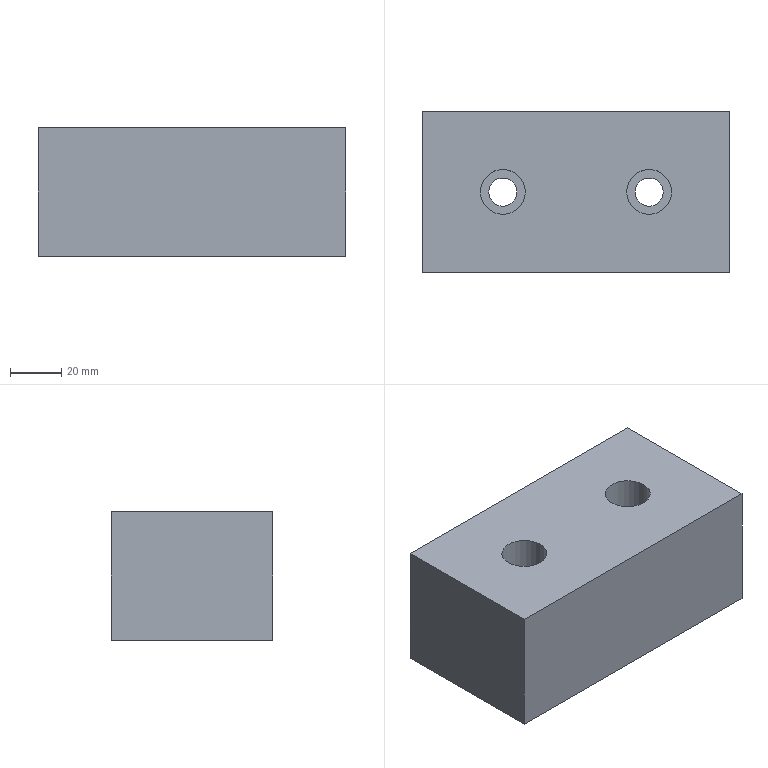Part | NX | features solid 2 | 1 solid | 12 faces | box 120 x 63 x 50 mm | volume 359767 mm3 | plane 8 | cylinder 4 | commonest cylinder face diameters 11 x2 17.5 x2
STEP:
#1=CARTESIAN_POINT('',(-1980.,-690.,-20.));
#2=VERTEX_POINT('',#1);
#3=CARTESIAN_POINT('',(-1980.,-627.,-20.));
#4=VERTEX_POINT('',#3);
#5=CARTESIAN_POINT('',(-1980.,-690.,-20.));
#6=DIRECTION('',(0.,1.,0.));
#7=VECTOR('',#6,1000.);
#8=LINE('',#5,#7);
#9=EDGE_CURVE('',#2,#4,#8,.T.);
#10=ORIENTED_EDGE('',*,*,#9,.F.);
#11=CARTESIAN_POINT('',(-1980.,-690.,30.));
#12=VERTEX_POINT('',#11);
#13=CARTESIAN_POINT('',(-1980.,-690.,50.));
#14=DIRECTION('',(0.,0.,-1.));
#15=VECTOR('',#14,1000.);
#16=LINE('',#13,#15);
#17=EDGE_CURVE('',#12,#2,#16,.T.);
#18=ORIENTED_EDGE('',*,*,#17,.F.);
#19=CARTESIAN_POINT('',(-1980.,-627.,30.));
#20=VERTEX_POINT('',#19);
#21=CARTESIAN_POINT('',(-1980.,-690.,30.));
#22=DIRECTION('',(0.,1.,0.));
#23=VECTOR('',#22,1000.);
#24=LINE('',#21,#23);
#25=EDGE_CURVE('',#12,#20,#24,.T.);
#26=ORIENTED_EDGE('',*,*,#25,.T.);
#27=CARTESIAN_POINT('',(-1980.,-627.,50.));
#28=DIRECTION('',(0.,0.,-1.));
#29=VECTOR('',#28,1000.);
#30=LINE('',#27,#29);
#31=EDGE_CURVE('',#20,#4,#30,.T.);
#32=ORIENTED_EDGE('',*,*,#31,.T.);
#33=EDGE_LOOP('',(#10,#18,#26,#32));
#34=FACE_BOUND('',#33,.T.);
#35=CARTESIAN_POINT('',(-1980.,-690.,50.));
#36=DIRECTION('',(-1.,0.,0.));
#37=DIRECTION('',(0.,-1.,0.));
#38=AXIS2_PLACEMENT_3D('',#35,#36,#37);
#39=PLANE('',#38);
#40=ADVANCED_FACE('',(#34),#39,.T.);
#41=CARTESIAN_POINT('',(-1860.,-627.,-20.));
#42=VERTEX_POINT('',#41);
#43=CARTESIAN_POINT('',(-1980.,-627.,-20.));
#44=DIRECTION('',(1.,0.,0.));
#45=VECTOR('',#44,1000.);
#46=LINE('',#43,#45);
#47=EDGE_CURVE('',#4,#42,#46,.T.);
#48=ORIENTED_EDGE('',*,*,#47,.F.);
#49=ORIENTED_EDGE('',*,*,#31,.F.);
#50=CARTESIAN_POINT('',(-1860.,-627.,30.));
#51=VERTEX_POINT('',#50);
#52=CARTESIAN_POINT('',(-1980.,-627.,30.));
#53=DIRECTION('',(1.,0.,0.));
#54=VECTOR('',#53,1000.);
#55=LINE('',#52,#54);
#56=EDGE_CURVE('',#20,#51,#55,.T.);
#57=ORIENTED_EDGE('',*,*,#56,.T.);
#58=CARTESIAN_POINT('',(-1860.,-627.,50.));
#59=DIRECTION('',(0.,0.,-1.));
#60=VECTOR('',#59,1000.);
#61=LINE('',#58,#60);
#62=EDGE_CURVE('',#51,#42,#61,.T.);
#63=ORIENTED_EDGE('',*,*,#62,.T.);
#64=EDGE_LOOP('',(#48,#49,#57,#63));
#65=FACE_BOUND('',#64,.T.);
#66=CARTESIAN_POINT('',(-1980.,-627.,50.));
#67=DIRECTION('',(0.,1.,0.));
#68=DIRECTION('',(0.,0.,1.));
#69=AXIS2_PLACEMENT_3D('',#66,#67,#68);
#70=PLANE('',#69);
#71=ADVANCED_FACE('',(#65),#70,.T.);
#72=CARTESIAN_POINT('',(-1860.,-690.,-20.));
#73=VERTEX_POINT('',#72);
#74=CARTESIAN_POINT('',(-1860.,-627.,-20.));
#75=DIRECTION('',(0.,-1.,0.));
#76=VECTOR('',#75,1000.);
#77=LINE('',#74,#76);
#78=EDGE_CURVE('',#42,#73,#77,.T.);
#79=ORIENTED_EDGE('',*,*,#78,.F.);
#80=ORIENTED_EDGE('',*,*,#62,.F.);
#81=CARTESIAN_POINT('',(-1860.,-690.,30.));
#82=VERTEX_POINT('',#81);
#83=CARTESIAN_POINT('',(-1860.,-627.,30.));
#84=DIRECTION('',(0.,-1.,0.));
#85=VECTOR('',#84,1000.);
#86=LINE('',#83,#85);
#87=EDGE_CURVE('',#51,#82,#86,.T.);
#88=ORIENTED_EDGE('',*,*,#87,.T.);
#89=CARTESIAN_POINT('',(-1860.,-690.,50.));
#90=DIRECTION('',(0.,0.,-1.));
#91=VECTOR('',#90,1000.);
#92=LINE('',#89,#91);
#93=EDGE_CURVE('',#82,#73,#92,.T.);
#94=ORIENTED_EDGE('',*,*,#93,.T.);
#95=EDGE_LOOP('',(#79,#80,#88,#94));
#96=FACE_BOUND('',#95,.T.);
#97=CARTESIAN_POINT('',(-1860.,-627.,50.));
#98=DIRECTION('',(1.,0.,0.));
#99=DIRECTION('',(0.,1.,0.));
#100=AXIS2_PLACEMENT_3D('',#97,#98,#99);
#101=PLANE('',#100);
#102=ADVANCED_FACE('',(#96),#101,.T.);
#103=CARTESIAN_POINT('',(-1860.,-690.,-20.));
#104=DIRECTION('',(-1.,0.,0.));
#105=VECTOR('',#104,1000.);
#106=LINE('',#103,#105);
#107=EDGE_CURVE('',#73,#2,#106,.T.);
#108=ORIENTED_EDGE('',*,*,#107,.F.);
#109=ORIENTED_EDGE('',*,*,#93,.F.);
#110=CARTESIAN_POINT('',(-1860.,-690.,30.));
#111=DIRECTION('',(-1.,0.,0.));
#112=VECTOR('',#111,1000.);
#113=LINE('',#110,#112);
#114=EDGE_CURVE('',#82,#12,#113,.T.);
#115=ORIENTED_EDGE('',*,*,#114,.T.);
#116=ORIENTED_EDGE('',*,*,#17,.T.);
#117=EDGE_LOOP('',(#108,#109,#115,#116));
#118=FACE_BOUND('',#117,.T.);
#119=CARTESIAN_POINT('',(-1860.,-690.,50.));
#120=DIRECTION('',(0.,-1.,0.));
#121=DIRECTION('',(1.,0.,0.));
#122=AXIS2_PLACEMENT_3D('',#119,#120,#121);
#123=PLANE('',#122);
#124=ADVANCED_FACE('',(#118),#123,.T.);
#125=CARTESIAN_POINT('',(-1957.25,-658.5,30.));
#126=VERTEX_POINT('',#125);
#127=CARTESIAN_POINT('',(-1948.5,-658.5,30.));
#128=DIRECTION('',(0.,0.,1.));
#129=DIRECTION('',(-1.,0.,0.));
#130=AXIS2_PLACEMENT_3D('',#127,#128,#129);
#131=CIRCLE('',#130,8.75);
#132=EDGE_CURVE('',#126,#126,#131,.T.);
#133=ORIENTED_EDGE('',*,*,#132,.F.);
#134=EDGE_LOOP('',(#133));
#135=FACE_BOUND('',#134,.T.);
#136=CARTESIAN_POINT('',(-1900.25,-658.5,30.));
#137=VERTEX_POINT('',#136);
#138=CARTESIAN_POINT('',(-1891.5,-658.5,30.));
#139=DIRECTION('',(0.,0.,1.));
#140=DIRECTION('',(-1.,0.,0.));
#141=AXIS2_PLACEMENT_3D('',#138,#139,#140);
#142=CIRCLE('',#141,8.75);
#143=EDGE_CURVE('',#137,#137,#142,.F.);
#144=ORIENTED_EDGE('',*,*,#143,.T.);
#145=EDGE_LOOP('',(#144));
#146=FACE_BOUND('',#145,.T.);
#147=ORIENTED_EDGE('',*,*,#25,.F.);
#148=ORIENTED_EDGE('',*,*,#114,.F.);
#149=ORIENTED_EDGE('',*,*,#87,.F.);
#150=ORIENTED_EDGE('',*,*,#56,.F.);
#151=EDGE_LOOP('',(#147,#148,#149,#150));
#152=FACE_BOUND('',#151,.T.);
#153=CARTESIAN_POINT('',(-1980.,-627.,30.));
#154=DIRECTION('',(0.,0.,-1.));
#155=DIRECTION('',(-1.,0.,0.));
#156=AXIS2_PLACEMENT_3D('',#153,#154,#155);
#157=PLANE('',#156);
#158=ADVANCED_FACE('',(#135,#146,#152),#157,.F.);
#159=CARTESIAN_POINT('',(-1954.,-658.5,-20.));
#160=VERTEX_POINT('',#159);
#161=CARTESIAN_POINT('',(-1948.5,-658.5,-20.));
#162=DIRECTION('',(0.,0.,-1.));
#163=DIRECTION('',(-1.,0.,0.));
#164=AXIS2_PLACEMENT_3D('',#161,#162,#163);
#165=CIRCLE('',#164,5.5);
#166=EDGE_CURVE('',#160,#160,#165,.T.);
#167=ORIENTED_EDGE('',*,*,#166,.F.);
#168=EDGE_LOOP('',(#167));
#169=FACE_BOUND('',#168,.T.);
#170=CARTESIAN_POINT('',(-1897.,-658.5,-20.));
#171=VERTEX_POINT('',#170);
#172=CARTESIAN_POINT('',(-1891.5,-658.5,-20.));
#173=DIRECTION('',(0.,0.,-1.));
#174=DIRECTION('',(-1.,0.,0.));
#175=AXIS2_PLACEMENT_3D('',#172,#173,#174);
#176=CIRCLE('',#175,5.5);
#177=EDGE_CURVE('',#171,#171,#176,.T.);
#178=ORIENTED_EDGE('',*,*,#177,.F.);
#179=EDGE_LOOP('',(#178));
#180=FACE_BOUND('',#179,.T.);
#181=ORIENTED_EDGE('',*,*,#9,.T.);
#182=ORIENTED_EDGE('',*,*,#47,.T.);
#183=ORIENTED_EDGE('',*,*,#78,.T.);
#184=ORIENTED_EDGE('',*,*,#107,.T.);
#185=EDGE_LOOP('',(#181,#182,#183,#184));
#186=FACE_BOUND('',#185,.T.);
#187=CARTESIAN_POINT('',(-1980.,-627.,-20.));
#188=DIRECTION('',(0.,0.,-1.));
#189=DIRECTION('',(-1.,0.,0.));
#190=AXIS2_PLACEMENT_3D('',#187,#188,#189);
#191=PLANE('',#190);
#192=ADVANCED_FACE('',(#169,#180,#186),#191,.T.);
#193=ORIENTED_EDGE('',*,*,#177,.T.);
#194=EDGE_LOOP('',(#193));
#195=FACE_BOUND('',#194,.T.);
#196=CARTESIAN_POINT('',(-1897.,-658.5,0.));
#197=VERTEX_POINT('',#196);
#198=CARTESIAN_POINT('',(-1891.5,-658.5,0.));
#199=DIRECTION('',(0.,0.,-1.));
#200=DIRECTION('',(-1.,0.,0.));
#201=AXIS2_PLACEMENT_3D('',#198,#199,#200);
#202=CIRCLE('',#201,5.5);
#203=EDGE_CURVE('',#197,#197,#202,.T.);
#204=ORIENTED_EDGE('',*,*,#203,.F.);
#205=EDGE_LOOP('',(#204));
#206=FACE_BOUND('',#205,.T.);
#207=CARTESIAN_POINT('',(-1891.5,-658.5,-60.));
#208=DIRECTION('',(0.,0.,-1.));
#209=DIRECTION('',(-1.,0.,0.));
#210=AXIS2_PLACEMENT_3D('',#207,#208,#209);
#211=CYLINDRICAL_SURFACE('',#210,5.5);
#212=ADVANCED_FACE('',(#195,#206),#211,.F.);
#213=ORIENTED_EDGE('',*,*,#203,.T.);
#214=EDGE_LOOP('',(#213));
#215=FACE_BOUND('',#214,.T.);
#216=CARTESIAN_POINT('',(-1900.25,-658.5,0.));
#217=VERTEX_POINT('',#216);
#218=CARTESIAN_POINT('',(-1891.5,-658.5,0.));
#219=DIRECTION('',(0.,0.,-1.));
#220=DIRECTION('',(-1.,0.,0.));
#221=AXIS2_PLACEMENT_3D('',#218,#219,#220);
#222=CIRCLE('',#221,8.75);
#223=EDGE_CURVE('',#217,#217,#222,.T.);
#224=ORIENTED_EDGE('',*,*,#223,.F.);
#225=EDGE_LOOP('',(#224));
#226=FACE_BOUND('',#225,.T.);
#227=CARTESIAN_POINT('',(-1891.5,-658.5,0.));
#228=DIRECTION('',(0.,0.,-1.));
#229=DIRECTION('',(-1.,0.,0.));
#230=AXIS2_PLACEMENT_3D('',#227,#228,#229);
#231=PLANE('',#230);
#232=ADVANCED_FACE('',(#215,#226),#231,.F.);
#233=ORIENTED_EDGE('',*,*,#223,.T.);
#234=EDGE_LOOP('',(#233));
#235=FACE_BOUND('',#234,.T.);
#236=ORIENTED_EDGE('',*,*,#143,.F.);
#237=EDGE_LOOP('',(#236));
#238=FACE_BOUND('',#237,.T.);
#239=CARTESIAN_POINT('',(-1891.5,-658.5,50.));
#240=DIRECTION('',(0.,0.,-1.));
#241=DIRECTION('',(-1.,0.,0.));
#242=AXIS2_PLACEMENT_3D('',#239,#240,#241);
#243=CYLINDRICAL_SURFACE('',#242,8.75);
#244=ADVANCED_FACE('',(#235,#238),#243,.F.);
#245=ORIENTED_EDGE('',*,*,#166,.T.);
#246=EDGE_LOOP('',(#245));
#247=FACE_BOUND('',#246,.T.);
#248=CARTESIAN_POINT('',(-1943.,-658.5,0.));
#249=VERTEX_POINT('',#248);
#250=CARTESIAN_POINT('',(-1948.5,-658.5,0.));
#251=DIRECTION('',(0.,0.,1.));
#252=DIRECTION('',(1.,0.,0.));
#253=AXIS2_PLACEMENT_3D('',#250,#251,#252);
#254=CIRCLE('',#253,5.5);
#255=EDGE_CURVE('',#249,#249,#254,.T.);
#256=ORIENTED_EDGE('',*,*,#255,.T.);
#257=EDGE_LOOP('',(#256));
#258=FACE_BOUND('',#257,.T.);
#259=CARTESIAN_POINT('',(-1948.5,-658.5,-60.));
#260=DIRECTION('',(0.,0.,-1.));
#261=DIRECTION('',(1.,0.,0.));
#262=AXIS2_PLACEMENT_3D('',#259,#260,#261);
#263=CYLINDRICAL_SURFACE('',#262,5.5);
#264=ADVANCED_FACE('',(#247,#258),#263,.F.);
#265=ORIENTED_EDGE('',*,*,#255,.F.);
#266=EDGE_LOOP('',(#265));
#267=FACE_BOUND('',#266,.T.);
#268=CARTESIAN_POINT('',(-1939.75,-658.5,0.));
#269=VERTEX_POINT('',#268);
#270=CARTESIAN_POINT('',(-1948.5,-658.5,0.));
#271=DIRECTION('',(0.,0.,1.));
#272=DIRECTION('',(1.,0.,0.));
#273=AXIS2_PLACEMENT_3D('',#270,#271,#272);
#274=CIRCLE('',#273,8.75);
#275=EDGE_CURVE('',#269,#269,#274,.T.);
#276=ORIENTED_EDGE('',*,*,#275,.T.);
#277=EDGE_LOOP('',(#276));
#278=FACE_BOUND('',#277,.T.);
#279=CARTESIAN_POINT('',(-1948.5,-658.5,0.));
#280=DIRECTION('',(0.,0.,-1.));
#281=DIRECTION('',(1.,0.,0.));
#282=AXIS2_PLACEMENT_3D('',#279,#280,#281);
#283=PLANE('',#282);
#284=ADVANCED_FACE('',(#267,#278),#283,.F.);
#285=ORIENTED_EDGE('',*,*,#275,.F.);
#286=EDGE_LOOP('',(#285));
#287=FACE_BOUND('',#286,.T.);
#288=ORIENTED_EDGE('',*,*,#132,.T.);
#289=EDGE_LOOP('',(#288));
#290=FACE_BOUND('',#289,.T.);
#291=CARTESIAN_POINT('',(-1948.5,-658.5,50.));
#292=DIRECTION('',(0.,0.,-1.));
#293=DIRECTION('',(1.,0.,0.));
#294=AXIS2_PLACEMENT_3D('',#291,#292,#293);
#295=CYLINDRICAL_SURFACE('',#294,8.75);
#296=ADVANCED_FACE('',(#287,#290),#295,.F.);
#297=CLOSED_SHELL('',(#40,#71,#102,#124,#158,#192,#212,#232,#244,#264,#284,#296));
#298=MANIFOLD_SOLID_BREP('',#297);
#299=(LENGTH_UNIT()NAMED_UNIT(*)SI_UNIT(.MILLI.,.METRE.));
#300=UNCERTAINTY_MEASURE_WITH_UNIT(LENGTH_MEASURE(0.00001),#299,'','');
#301=(NAMED_UNIT(*)PLANE_ANGLE_UNIT()SI_UNIT($,.RADIAN.));
#302=(NAMED_UNIT(*)SI_UNIT($,.STERADIAN.)SOLID_ANGLE_UNIT());
#303=(GEOMETRIC_REPRESENTATION_CONTEXT(3)GLOBAL_UNCERTAINTY_ASSIGNED_CONTEXT((#300))GLOBAL_UNIT_ASSIGNED_CONTEXT((#299,#301,#302))REPRESENTATION_CONTEXT('',''));
#304=ADVANCED_BREP_SHAPE_REPRESENTATION('',(#298),#303);